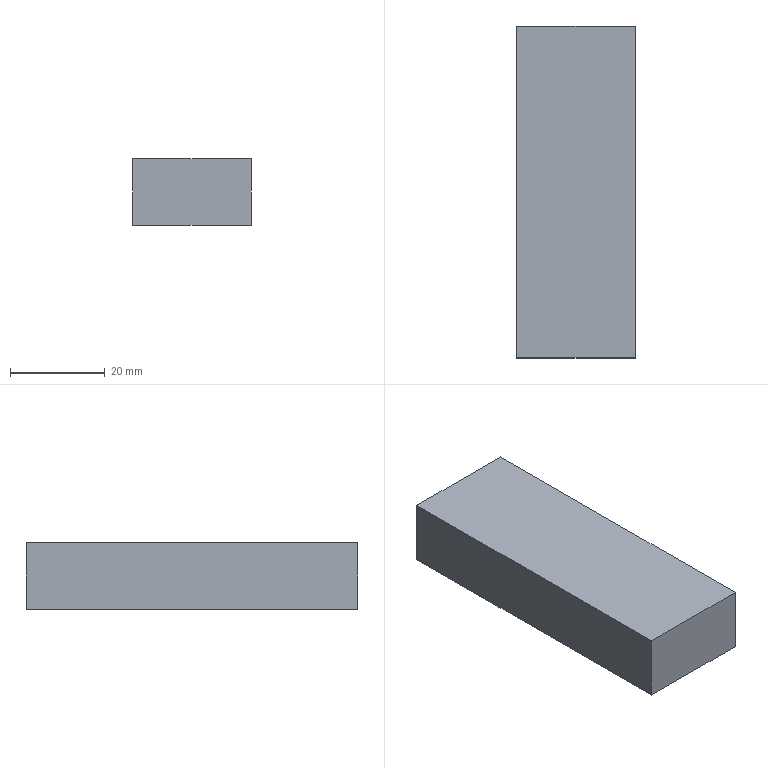Part | SolidWorks | features Extrusion 1 | 1 solid | 6 faces | box 25 x 70 x 14 mm | volume 24500 mm3 | plane 6
STEP:
#1=CARTESIAN_POINT('',(12.5,-35.,-7.));
#2=VERTEX_POINT('',#1);
#3=CARTESIAN_POINT('',(12.5,35.,-7.));
#4=VERTEX_POINT('',#3);
#5=CARTESIAN_POINT('',(12.5,-35.,-7.));
#6=DIRECTION('',(0.,1.,0.));
#7=VECTOR('',#6,1000.);
#8=LINE('',#5,#7);
#9=EDGE_CURVE('',#2,#4,#8,.T.);
#10=ORIENTED_EDGE('',*,*,#9,.T.);
#11=CARTESIAN_POINT('',(12.5,35.,7.));
#12=VERTEX_POINT('',#11);
#13=CARTESIAN_POINT('',(12.5,35.,7.));
#14=DIRECTION('',(0.,0.,-1.));
#15=VECTOR('',#14,1000.);
#16=LINE('',#13,#15);
#17=EDGE_CURVE('',#12,#4,#16,.T.);
#18=ORIENTED_EDGE('',*,*,#17,.F.);
#19=CARTESIAN_POINT('',(12.5,-35.,7.));
#20=VERTEX_POINT('',#19);
#21=CARTESIAN_POINT('',(12.5,-35.,7.));
#22=DIRECTION('',(0.,1.,0.));
#23=VECTOR('',#22,1000.);
#24=LINE('',#21,#23);
#25=EDGE_CURVE('',#20,#12,#24,.T.);
#26=ORIENTED_EDGE('',*,*,#25,.F.);
#27=CARTESIAN_POINT('',(12.5,-35.,7.));
#28=DIRECTION('',(0.,0.,-1.));
#29=VECTOR('',#28,1000.);
#30=LINE('',#27,#29);
#31=EDGE_CURVE('',#20,#2,#30,.T.);
#32=ORIENTED_EDGE('',*,*,#31,.T.);
#33=EDGE_LOOP('',(#10,#18,#26,#32));
#34=FACE_OUTER_BOUND('',#33,.T.);
#35=CARTESIAN_POINT('',(12.5,-35.,7.));
#36=DIRECTION('',(-1.,0.,0.));
#37=DIRECTION('',(0.,0.,1.));
#38=AXIS2_PLACEMENT_3D('',#35,#36,#37);
#39=PLANE('',#38);
#40=ADVANCED_FACE('',(#34),#39,.F.);
#41=CARTESIAN_POINT('',(-12.5,35.,-7.));
#42=VERTEX_POINT('',#41);
#43=CARTESIAN_POINT('',(-12.5,35.,-7.));
#44=DIRECTION('',(-1.,0.,0.));
#45=VECTOR('',#44,1000.);
#46=LINE('',#43,#45);
#47=EDGE_CURVE('',#4,#42,#46,.T.);
#48=ORIENTED_EDGE('',*,*,#47,.T.);
#49=CARTESIAN_POINT('',(-12.5,35.,7.));
#50=VERTEX_POINT('',#49);
#51=CARTESIAN_POINT('',(-12.5,35.,7.));
#52=DIRECTION('',(0.,0.,-1.));
#53=VECTOR('',#52,1000.);
#54=LINE('',#51,#53);
#55=EDGE_CURVE('',#50,#42,#54,.T.);
#56=ORIENTED_EDGE('',*,*,#55,.F.);
#57=CARTESIAN_POINT('',(-12.5,35.,7.));
#58=DIRECTION('',(-1.,0.,0.));
#59=VECTOR('',#58,1000.);
#60=LINE('',#57,#59);
#61=EDGE_CURVE('',#12,#50,#60,.T.);
#62=ORIENTED_EDGE('',*,*,#61,.F.);
#63=ORIENTED_EDGE('',*,*,#17,.T.);
#64=EDGE_LOOP('',(#48,#56,#62,#63));
#65=FACE_OUTER_BOUND('',#64,.T.);
#66=CARTESIAN_POINT('',(-12.5,35.,7.));
#67=DIRECTION('',(0.,-1.,0.));
#68=DIRECTION('',(0.,0.,-1.));
#69=AXIS2_PLACEMENT_3D('',#66,#67,#68);
#70=PLANE('',#69);
#71=ADVANCED_FACE('',(#65),#70,.F.);
#72=CARTESIAN_POINT('',(-12.5,-35.,-7.));
#73=VERTEX_POINT('',#72);
#74=CARTESIAN_POINT('',(-12.5,-35.,-7.));
#75=DIRECTION('',(0.,-1.,0.));
#76=VECTOR('',#75,1000.);
#77=LINE('',#74,#76);
#78=EDGE_CURVE('',#42,#73,#77,.T.);
#79=ORIENTED_EDGE('',*,*,#78,.T.);
#80=CARTESIAN_POINT('',(-12.5,-35.,7.));
#81=VERTEX_POINT('',#80);
#82=CARTESIAN_POINT('',(-12.5,-35.,7.));
#83=DIRECTION('',(0.,0.,-1.));
#84=VECTOR('',#83,1000.);
#85=LINE('',#82,#84);
#86=EDGE_CURVE('',#81,#73,#85,.T.);
#87=ORIENTED_EDGE('',*,*,#86,.F.);
#88=CARTESIAN_POINT('',(-12.5,-35.,7.));
#89=DIRECTION('',(0.,-1.,0.));
#90=VECTOR('',#89,1000.);
#91=LINE('',#88,#90);
#92=EDGE_CURVE('',#50,#81,#91,.T.);
#93=ORIENTED_EDGE('',*,*,#92,.F.);
#94=ORIENTED_EDGE('',*,*,#55,.T.);
#95=EDGE_LOOP('',(#79,#87,#93,#94));
#96=FACE_OUTER_BOUND('',#95,.T.);
#97=CARTESIAN_POINT('',(-12.5,-35.,7.));
#98=DIRECTION('',(1.,0.,0.));
#99=DIRECTION('',(0.,0.,-1.));
#100=AXIS2_PLACEMENT_3D('',#97,#98,#99);
#101=PLANE('',#100);
#102=ADVANCED_FACE('',(#96),#101,.F.);
#103=CARTESIAN_POINT('',(-12.5,-35.,-7.));
#104=DIRECTION('',(1.,0.,0.));
#105=VECTOR('',#104,1000.);
#106=LINE('',#103,#105);
#107=EDGE_CURVE('',#73,#2,#106,.T.);
#108=ORIENTED_EDGE('',*,*,#107,.T.);
#109=ORIENTED_EDGE('',*,*,#31,.F.);
#110=CARTESIAN_POINT('',(-12.5,-35.,7.));
#111=DIRECTION('',(1.,0.,0.));
#112=VECTOR('',#111,1000.);
#113=LINE('',#110,#112);
#114=EDGE_CURVE('',#81,#20,#113,.T.);
#115=ORIENTED_EDGE('',*,*,#114,.F.);
#116=ORIENTED_EDGE('',*,*,#86,.T.);
#117=EDGE_LOOP('',(#108,#109,#115,#116));
#118=FACE_OUTER_BOUND('',#117,.T.);
#119=CARTESIAN_POINT('',(-12.5,-35.,7.));
#120=DIRECTION('',(0.,1.,0.));
#121=DIRECTION('',(0.,0.,1.));
#122=AXIS2_PLACEMENT_3D('',#119,#120,#121);
#123=PLANE('',#122);
#124=ADVANCED_FACE('',(#118),#123,.F.);
#125=ORIENTED_EDGE('',*,*,#25,.T.);
#126=ORIENTED_EDGE('',*,*,#61,.T.);
#127=ORIENTED_EDGE('',*,*,#92,.T.);
#128=ORIENTED_EDGE('',*,*,#114,.T.);
#129=EDGE_LOOP('',(#125,#126,#127,#128));
#130=FACE_OUTER_BOUND('',#129,.T.);
#131=CARTESIAN_POINT('',(0.,0.,7.));
#132=DIRECTION('',(0.,0.,-1.));
#133=DIRECTION('',(-1.,0.,0.));
#134=AXIS2_PLACEMENT_3D('',#131,#132,#133);
#135=PLANE('',#134);
#136=ADVANCED_FACE('',(#130),#135,.F.);
#137=ORIENTED_EDGE('',*,*,#9,.F.);
#138=ORIENTED_EDGE('',*,*,#107,.F.);
#139=ORIENTED_EDGE('',*,*,#78,.F.);
#140=ORIENTED_EDGE('',*,*,#47,.F.);
#141=EDGE_LOOP('',(#137,#138,#139,#140));
#142=FACE_OUTER_BOUND('',#141,.T.);
#143=CARTESIAN_POINT('',(0.,0.,-7.));
#144=DIRECTION('',(0.,0.,-1.));
#145=DIRECTION('',(-1.,0.,0.));
#146=AXIS2_PLACEMENT_3D('',#143,#144,#145);
#147=PLANE('',#146);
#148=ADVANCED_FACE('',(#142),#147,.T.);
#149=CLOSED_SHELL('',(#40,#71,#102,#124,#136,#148));
#150=MANIFOLD_SOLID_BREP('',#149);
#151=CARTESIAN_POINT('',(0.,0.,0.));
#152=DIRECTION('',(0.,0.,1.));
#153=DIRECTION('',(1.,0.,0.));
#154=AXIS2_PLACEMENT_3D('',#151,#152,#153);
#155=(LENGTH_UNIT()NAMED_UNIT(*)SI_UNIT(.MILLI.,.METRE.));
#156=UNCERTAINTY_MEASURE_WITH_UNIT(LENGTH_MEASURE(0.00001),#155,'','');
#157=(NAMED_UNIT(*)PLANE_ANGLE_UNIT()SI_UNIT($,.RADIAN.));
#158=(NAMED_UNIT(*)SI_UNIT($,.STERADIAN.)SOLID_ANGLE_UNIT());
#159=(GEOMETRIC_REPRESENTATION_CONTEXT(3)GLOBAL_UNCERTAINTY_ASSIGNED_CONTEXT((#156))GLOBAL_UNIT_ASSIGNED_CONTEXT((#155,#157,#158))REPRESENTATION_CONTEXT('',''));
#160=ADVANCED_BREP_SHAPE_REPRESENTATION('',(#150,#154),#159);